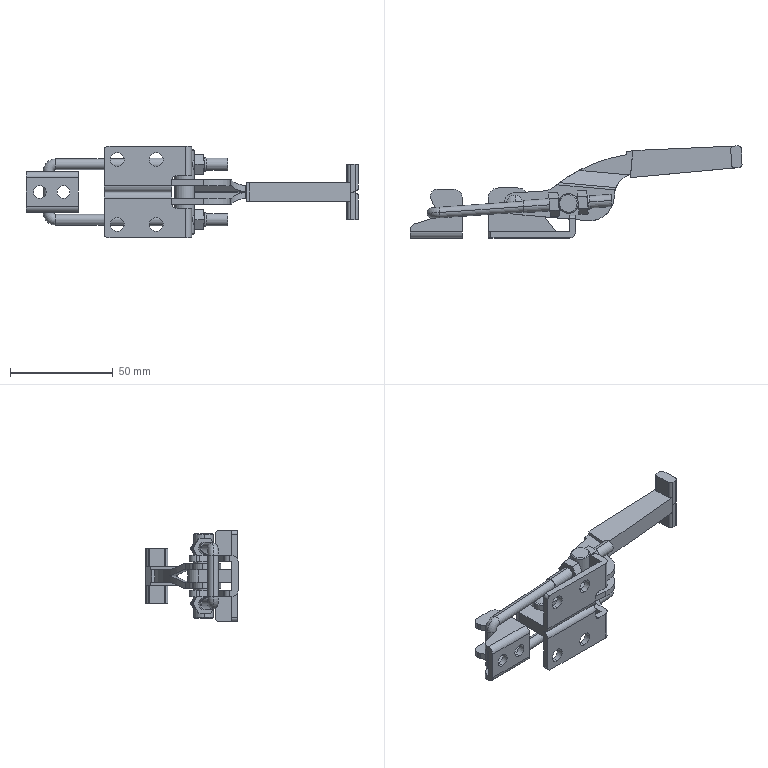Part | SolidWorks | 5 solids | 230 faces | box 161.788 x 44.909 x 44.4 mm | volume 32694 mm3 | plane 110 | cylinder 104 | torus 10 | cone 4 | sphere 2 | commonest cylinder face diameters 6 x24 3 x11 4 x8 6.7 x8 7 x8 5.2 x6